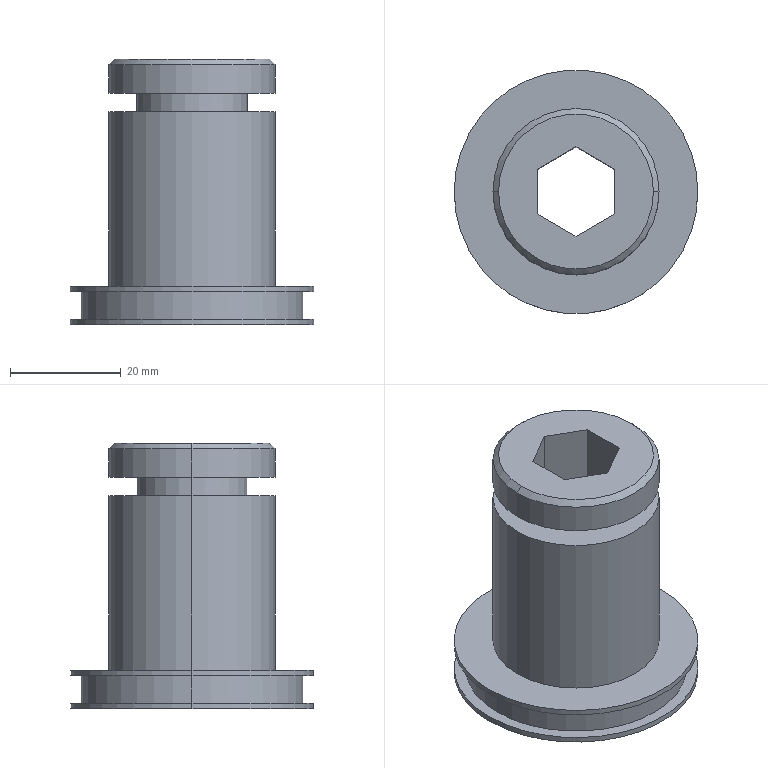Part | STEP file | 103-01-0006 | 1 solid | 27 faces | box 44 x 44 x 48 mm | volume 28816 mm3 | plane 13 | cylinder 12 | cone 2 | commonest cylinder face diameters 30 x4 44 x4 20 x2 40 x2